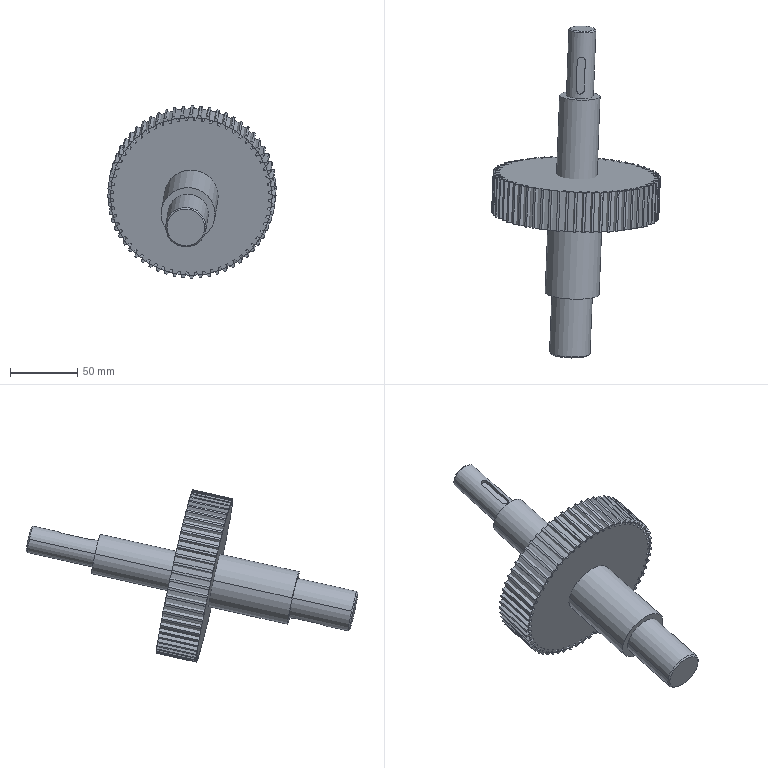Part | SolidWorks | 1 solid | 272 faces | box 125.053 x 245.99 x 127.556 mm | volume 298117 mm3 | cylinder 255 | plane 13 | cone 4 | commonest cylinder face diameters 50.476 x120 124 x61 115 x60 30 x4 6 x2 8 x2